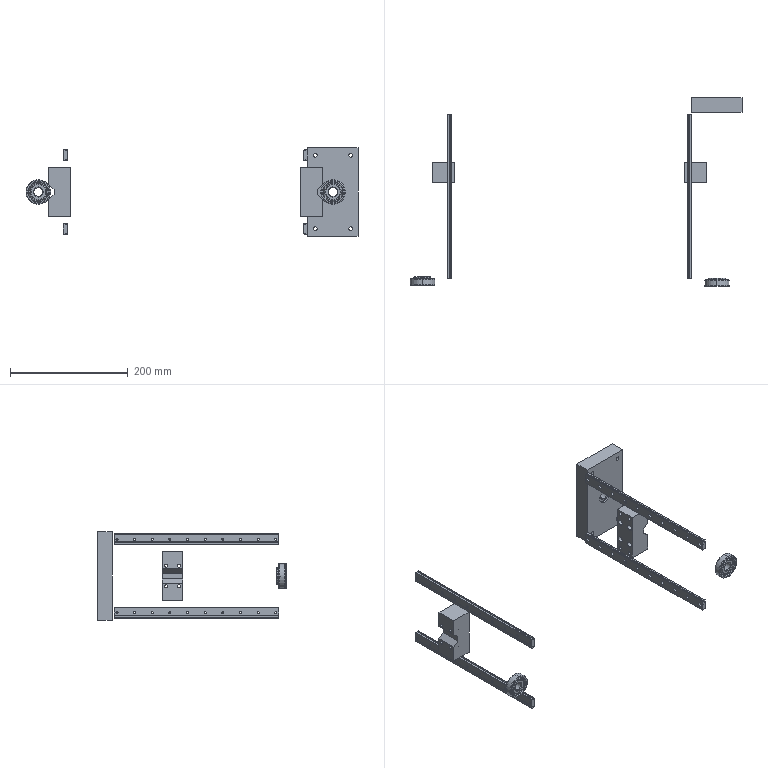Part | NX | features BREP 17 | 34 solids | 773 faces | box 564.5 x 321 x 150 mm | volume 641076 mm3 | cylinder 314 | plane 187 | torus 124 | sphere 96 | cone 52 | commonest cylinder face diameters 6.5 x104 3.5 x80 5.563 x40 5.5 x16 9.5 x16 2 x12